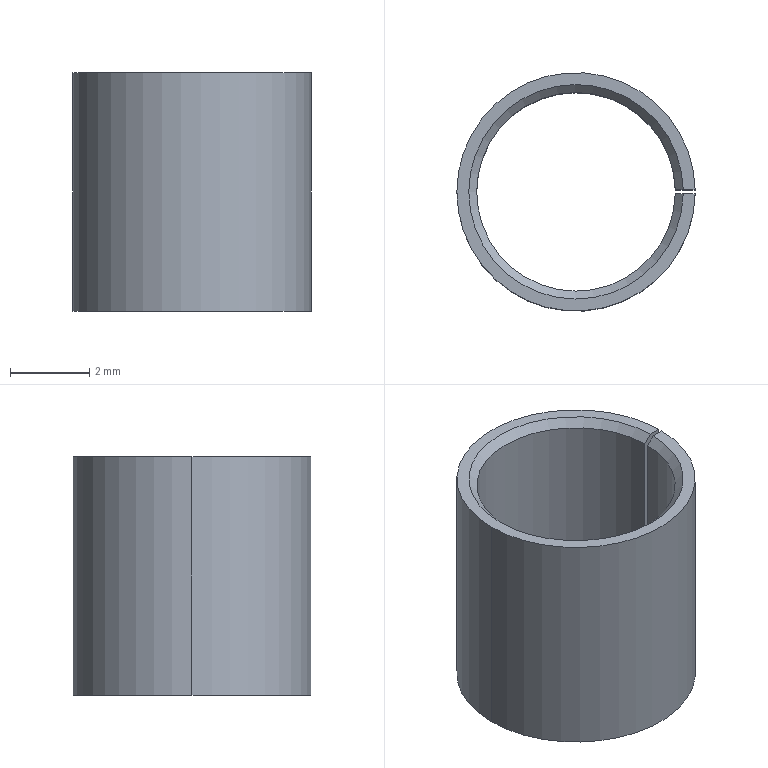Part | SolidWorks | features Chamfer 1, Extrusion 1, ICE 1 | 1 solid | 11 faces | box 6 x 6 x 6 mm | volume 50.895 mm3 | cylinder 4 | plane 4 | cone 3 | commonest cylinder face diameters 5 x2 6 x2
STEP:
#1=CARTESIAN_POINT('',(-2.5,0.,0.2));
#2=VERTEX_POINT('',#1);
#3=CARTESIAN_POINT('',(2.499,0.05,0.2));
#4=VERTEX_POINT('',#3);
#5=CARTESIAN_POINT('',(0.,0.,0.2));
#6=DIRECTION('',(0.,0.,-1.));
#7=DIRECTION('',(1.,0.,0.));
#8=AXIS2_PLACEMENT_3D('',#5,#6,#7);
#9=CIRCLE('',#8,2.5);
#10=EDGE_CURVE('',#2,#4,#9,.T.);
#11=ORIENTED_EDGE('',*,*,#10,.F.);
#12=CARTESIAN_POINT('',(-2.7,0.,0.));
#13=VERTEX_POINT('',#12);
#14=CARTESIAN_POINT('',(-2.7,0.,0.));
#15=DIRECTION('',(-0.7071,0.,-0.7071));
#16=VECTOR('',#15,1000.);
#17=LINE('',#14,#16);
#18=EDGE_CURVE('',#2,#13,#17,.T.);
#19=ORIENTED_EDGE('',*,*,#18,.T.);
#20=CARTESIAN_POINT('',(2.7,0.05,0.));
#21=VERTEX_POINT('',#20);
#22=CARTESIAN_POINT('',(0.,0.,0.));
#23=DIRECTION('',(0.,0.,1.));
#24=DIRECTION('',(1.,0.,0.));
#25=AXIS2_PLACEMENT_3D('',#22,#23,#24);
#26=CIRCLE('',#25,2.7);
#27=EDGE_CURVE('',#21,#13,#26,.T.);
#28=ORIENTED_EDGE('',*,*,#27,.F.);
#29=CARTESIAN_POINT('',(2.499,0.05,0.2));
#30=CARTESIAN_POINT('',(2.566,0.05,0.1333));
#31=CARTESIAN_POINT('',(2.633,0.05,0.06667));
#32=CARTESIAN_POINT('',(2.7,0.05,0.));
#33=B_SPLINE_CURVE_WITH_KNOTS('',3,(#29,#30,#31,#32),.UNSPECIFIED.,.F.,.F.,(4,4),(0.002926,0.003209),.UNSPECIFIED.);
#34=EDGE_CURVE('',#4,#21,#33,.T.);
#35=ORIENTED_EDGE('',*,*,#34,.F.);
#36=EDGE_LOOP('',(#11,#19,#28,#35));
#37=FACE_OUTER_BOUND('',#36,.T.);
#38=CARTESIAN_POINT('',(0.,0.,0.));
#39=DIRECTION('',(0.,0.,-1.));
#40=DIRECTION('',(-1.,0.,0.));
#41=AXIS2_PLACEMENT_3D('',#38,#39,#40);
#42=CONICAL_SURFACE('',#41,2.7,0.7854);
#43=ADVANCED_FACE('',(#37),#42,.F.);
#44=CARTESIAN_POINT('',(2.499,0.05,5.8));
#45=VERTEX_POINT('',#44);
#46=CARTESIAN_POINT('',(-2.5,0.,5.8));
#47=VERTEX_POINT('',#46);
#48=CARTESIAN_POINT('',(0.,0.,5.8));
#49=DIRECTION('',(0.,0.,1.));
#50=DIRECTION('',(1.,0.,0.));
#51=AXIS2_PLACEMENT_3D('',#48,#49,#50);
#52=CIRCLE('',#51,2.5);
#53=EDGE_CURVE('',#45,#47,#52,.T.);
#54=ORIENTED_EDGE('',*,*,#53,.T.);
#55=CARTESIAN_POINT('',(-2.5,0.,6.));
#56=DIRECTION('',(0.,0.,-1.));
#57=VECTOR('',#56,1000.);
#58=LINE('',#55,#57);
#59=EDGE_CURVE('',#47,#2,#58,.T.);
#60=ORIENTED_EDGE('',*,*,#59,.T.);
#61=ORIENTED_EDGE('',*,*,#10,.T.);
#62=CARTESIAN_POINT('',(2.499,0.05,6.));
#63=DIRECTION('',(0.,0.,-1.));
#64=VECTOR('',#63,1000.);
#65=LINE('',#62,#64);
#66=EDGE_CURVE('',#45,#4,#65,.T.);
#67=ORIENTED_EDGE('',*,*,#66,.F.);
#68=EDGE_LOOP('',(#54,#60,#61,#67));
#69=FACE_OUTER_BOUND('',#68,.T.);
#70=CARTESIAN_POINT('',(0.,0.,6.));
#71=DIRECTION('',(0.,0.,-1.));
#72=DIRECTION('',(-1.,0.,0.));
#73=AXIS2_PLACEMENT_3D('',#70,#71,#72);
#74=CYLINDRICAL_SURFACE('',#73,2.5);
#75=ADVANCED_FACE('',(#69),#74,.F.);
#76=CARTESIAN_POINT('',(-3.,0.,6.));
#77=VERTEX_POINT('',#76);
#78=CARTESIAN_POINT('',(3.,-0.05,6.));
#79=VERTEX_POINT('',#78);
#80=CARTESIAN_POINT('',(0.,0.,6.));
#81=DIRECTION('',(0.,0.,1.));
#82=DIRECTION('',(1.,0.,0.));
#83=AXIS2_PLACEMENT_3D('',#80,#81,#82);
#84=CIRCLE('',#83,3.);
#85=EDGE_CURVE('',#77,#79,#84,.T.);
#86=ORIENTED_EDGE('',*,*,#85,.F.);
#87=CARTESIAN_POINT('',(-3.,0.,0.));
#88=VERTEX_POINT('',#87);
#89=CARTESIAN_POINT('',(-3.,0.,6.));
#90=DIRECTION('',(0.,0.,-1.));
#91=VECTOR('',#90,1000.);
#92=LINE('',#89,#91);
#93=EDGE_CURVE('',#77,#88,#92,.T.);
#94=ORIENTED_EDGE('',*,*,#93,.T.);
#95=CARTESIAN_POINT('',(3.,-0.05,0.));
#96=VERTEX_POINT('',#95);
#97=CARTESIAN_POINT('',(0.,0.,0.));
#98=DIRECTION('',(0.,0.,1.));
#99=DIRECTION('',(1.,0.,0.));
#100=AXIS2_PLACEMENT_3D('',#97,#98,#99);
#101=CIRCLE('',#100,3.);
#102=EDGE_CURVE('',#88,#96,#101,.T.);
#103=ORIENTED_EDGE('',*,*,#102,.T.);
#104=CARTESIAN_POINT('',(3.,-0.05,6.));
#105=DIRECTION('',(0.,0.,1.));
#106=VECTOR('',#105,1000.);
#107=LINE('',#104,#106);
#108=EDGE_CURVE('',#96,#79,#107,.T.);
#109=ORIENTED_EDGE('',*,*,#108,.T.);
#110=EDGE_LOOP('',(#86,#94,#103,#109));
#111=FACE_OUTER_BOUND('',#110,.T.);
#112=CARTESIAN_POINT('',(0.,0.,6.));
#113=DIRECTION('',(0.,0.,-1.));
#114=DIRECTION('',(-1.,0.,0.));
#115=AXIS2_PLACEMENT_3D('',#112,#113,#114);
#116=CYLINDRICAL_SURFACE('',#115,3.);
#117=ADVANCED_FACE('',(#111),#116,.T.);
#118=CARTESIAN_POINT('',(2.7,-0.05,6.));
#119=VERTEX_POINT('',#118);
#120=CARTESIAN_POINT('',(0.6418,-0.05,6.));
#121=DIRECTION('',(1.,0.,0.));
#122=VECTOR('',#121,1000.);
#123=LINE('',#120,#122);
#124=EDGE_CURVE('',#119,#79,#123,.T.);
#125=ORIENTED_EDGE('',*,*,#124,.F.);
#126=CARTESIAN_POINT('',(2.7,0.05,6.));
#127=VERTEX_POINT('',#126);
#128=CARTESIAN_POINT('',(0.,0.,6.));
#129=DIRECTION('',(0.,0.,-1.));
#130=DIRECTION('',(1.,0.,0.));
#131=AXIS2_PLACEMENT_3D('',#128,#129,#130);
#132=CIRCLE('',#131,2.7);
#133=EDGE_CURVE('',#119,#127,#132,.T.);
#134=ORIENTED_EDGE('',*,*,#133,.T.);
#135=CARTESIAN_POINT('',(3.,0.05,6.));
#136=VERTEX_POINT('',#135);
#137=CARTESIAN_POINT('',(0.6418,0.05,6.));
#138=DIRECTION('',(-1.,0.,0.));
#139=VECTOR('',#138,1000.);
#140=LINE('',#137,#139);
#141=EDGE_CURVE('',#136,#127,#140,.T.);
#142=ORIENTED_EDGE('',*,*,#141,.F.);
#143=CARTESIAN_POINT('',(0.,0.,6.));
#144=DIRECTION('',(0.,0.,1.));
#145=DIRECTION('',(1.,0.,0.));
#146=AXIS2_PLACEMENT_3D('',#143,#144,#145);
#147=CIRCLE('',#146,3.);
#148=EDGE_CURVE('',#136,#77,#147,.T.);
#149=ORIENTED_EDGE('',*,*,#148,.T.);
#150=ORIENTED_EDGE('',*,*,#85,.T.);
#151=EDGE_LOOP('',(#125,#134,#142,#149,#150));
#152=FACE_OUTER_BOUND('',#151,.T.);
#153=CARTESIAN_POINT('',(0.,0.,6.));
#154=DIRECTION('',(0.,0.,1.));
#155=DIRECTION('',(1.,0.,0.));
#156=AXIS2_PLACEMENT_3D('',#153,#154,#155);
#157=PLANE('',#156);
#158=ADVANCED_FACE('',(#152),#157,.T.);
#159=ORIENTED_EDGE('',*,*,#27,.T.);
#160=CARTESIAN_POINT('',(2.7,-0.05,0.));
#161=VERTEX_POINT('',#160);
#162=CARTESIAN_POINT('',(0.,0.,0.));
#163=DIRECTION('',(0.,0.,1.));
#164=DIRECTION('',(1.,0.,0.));
#165=AXIS2_PLACEMENT_3D('',#162,#163,#164);
#166=CIRCLE('',#165,2.7);
#167=EDGE_CURVE('',#13,#161,#166,.T.);
#168=ORIENTED_EDGE('',*,*,#167,.T.);
#169=CARTESIAN_POINT('',(0.6418,-0.05,0.));
#170=DIRECTION('',(1.,0.,0.));
#171=VECTOR('',#170,1000.);
#172=LINE('',#169,#171);
#173=EDGE_CURVE('',#161,#96,#172,.T.);
#174=ORIENTED_EDGE('',*,*,#173,.T.);
#175=ORIENTED_EDGE('',*,*,#102,.F.);
#176=CARTESIAN_POINT('',(3.,0.05,0.));
#177=VERTEX_POINT('',#176);
#178=CARTESIAN_POINT('',(0.,0.,0.));
#179=DIRECTION('',(0.,0.,1.));
#180=DIRECTION('',(1.,0.,0.));
#181=AXIS2_PLACEMENT_3D('',#178,#179,#180);
#182=CIRCLE('',#181,3.);
#183=EDGE_CURVE('',#177,#88,#182,.T.);
#184=ORIENTED_EDGE('',*,*,#183,.F.);
#185=CARTESIAN_POINT('',(0.6418,0.05,0.));
#186=DIRECTION('',(-1.,0.,0.));
#187=VECTOR('',#186,1000.);
#188=LINE('',#185,#187);
#189=EDGE_CURVE('',#177,#21,#188,.T.);
#190=ORIENTED_EDGE('',*,*,#189,.T.);
#191=EDGE_LOOP('',(#159,#168,#174,#175,#184,#190));
#192=FACE_OUTER_BOUND('',#191,.T.);
#193=CARTESIAN_POINT('',(0.,0.,0.));
#194=DIRECTION('',(0.,0.,1.));
#195=DIRECTION('',(1.,0.,0.));
#196=AXIS2_PLACEMENT_3D('',#193,#194,#195);
#197=PLANE('',#196);
#198=ADVANCED_FACE('',(#192),#197,.F.);
#199=ORIENTED_EDGE('',*,*,#93,.F.);
#200=ORIENTED_EDGE('',*,*,#148,.F.);
#201=CARTESIAN_POINT('',(3.,0.05,6.));
#202=DIRECTION('',(0.,0.,-1.));
#203=VECTOR('',#202,1000.);
#204=LINE('',#201,#203);
#205=EDGE_CURVE('',#136,#177,#204,.T.);
#206=ORIENTED_EDGE('',*,*,#205,.T.);
#207=ORIENTED_EDGE('',*,*,#183,.T.);
#208=EDGE_LOOP('',(#199,#200,#206,#207));
#209=FACE_OUTER_BOUND('',#208,.T.);
#210=CARTESIAN_POINT('',(0.,0.,6.));
#211=DIRECTION('',(0.,0.,-1.));
#212=DIRECTION('',(-1.,0.,0.));
#213=AXIS2_PLACEMENT_3D('',#210,#211,#212);
#214=CYLINDRICAL_SURFACE('',#213,3.);
#215=ADVANCED_FACE('',(#209),#214,.T.);
#216=ORIENTED_EDGE('',*,*,#59,.F.);
#217=CARTESIAN_POINT('',(2.499,-0.05,5.8));
#218=VERTEX_POINT('',#217);
#219=CARTESIAN_POINT('',(0.,0.,5.8));
#220=DIRECTION('',(0.,0.,1.));
#221=DIRECTION('',(1.,0.,0.));
#222=AXIS2_PLACEMENT_3D('',#219,#220,#221);
#223=CIRCLE('',#222,2.5);
#224=EDGE_CURVE('',#47,#218,#223,.T.);
#225=ORIENTED_EDGE('',*,*,#224,.T.);
#226=CARTESIAN_POINT('',(2.499,-0.05,0.2));
#227=VERTEX_POINT('',#226);
#228=CARTESIAN_POINT('',(2.499,-0.05,6.));
#229=DIRECTION('',(0.,0.,1.));
#230=VECTOR('',#229,1000.);
#231=LINE('',#228,#230);
#232=EDGE_CURVE('',#227,#218,#231,.T.);
#233=ORIENTED_EDGE('',*,*,#232,.F.);
#234=CARTESIAN_POINT('',(0.,0.,0.2));
#235=DIRECTION('',(0.,0.,-1.));
#236=DIRECTION('',(1.,0.,0.));
#237=AXIS2_PLACEMENT_3D('',#234,#235,#236);
#238=CIRCLE('',#237,2.5);
#239=EDGE_CURVE('',#227,#2,#238,.T.);
#240=ORIENTED_EDGE('',*,*,#239,.T.);
#241=EDGE_LOOP('',(#216,#225,#233,#240));
#242=FACE_OUTER_BOUND('',#241,.T.);
#243=CARTESIAN_POINT('',(0.,0.,6.));
#244=DIRECTION('',(0.,0.,-1.));
#245=DIRECTION('',(-1.,0.,0.));
#246=AXIS2_PLACEMENT_3D('',#243,#244,#245);
#247=CYLINDRICAL_SURFACE('',#246,2.5);
#248=ADVANCED_FACE('',(#242),#247,.F.);
#249=ORIENTED_EDGE('',*,*,#18,.F.);
#250=ORIENTED_EDGE('',*,*,#239,.F.);
#251=CARTESIAN_POINT('',(2.7,-0.05,0.));
#252=CARTESIAN_POINT('',(2.633,-0.05,0.06667));
#253=CARTESIAN_POINT('',(2.566,-0.05,0.1333));
#254=CARTESIAN_POINT('',(2.499,-0.05,0.2));
#255=B_SPLINE_CURVE_WITH_KNOTS('',3,(#251,#252,#253,#254),.UNSPECIFIED.,.F.,.F.,(4,4),(0.002925,0.003208),.UNSPECIFIED.);
#256=EDGE_CURVE('',#161,#227,#255,.T.);
#257=ORIENTED_EDGE('',*,*,#256,.F.);
#258=ORIENTED_EDGE('',*,*,#167,.F.);
#259=EDGE_LOOP('',(#249,#250,#257,#258));
#260=FACE_OUTER_BOUND('',#259,.T.);
#261=CARTESIAN_POINT('',(0.,0.,0.));
#262=DIRECTION('',(0.,0.,-1.));
#263=DIRECTION('',(-1.,0.,0.));
#264=AXIS2_PLACEMENT_3D('',#261,#262,#263);
#265=CONICAL_SURFACE('',#264,2.7,0.7854);
#266=ADVANCED_FACE('',(#260),#265,.F.);
#267=CARTESIAN_POINT('',(2.499,-0.05,5.8));
#268=CARTESIAN_POINT('',(2.566,-0.05,5.867));
#269=CARTESIAN_POINT('',(2.633,-0.05,5.933));
#270=CARTESIAN_POINT('',(2.7,-0.05,6.));
#271=B_SPLINE_CURVE_WITH_KNOTS('',3,(#267,#268,#269,#270),.UNSPECIFIED.,.F.,.F.,(4,4),(0.002926,0.003209),.UNSPECIFIED.);
#272=EDGE_CURVE('',#218,#119,#271,.T.);
#273=ORIENTED_EDGE('',*,*,#272,.F.);
#274=ORIENTED_EDGE('',*,*,#224,.F.);
#275=ORIENTED_EDGE('',*,*,#53,.F.);
#276=CARTESIAN_POINT('',(2.7,0.05,6.));
#277=CARTESIAN_POINT('',(2.633,0.05,5.933));
#278=CARTESIAN_POINT('',(2.566,0.05,5.867));
#279=CARTESIAN_POINT('',(2.499,0.05,5.8));
#280=B_SPLINE_CURVE_WITH_KNOTS('',3,(#276,#277,#278,#279),.UNSPECIFIED.,.F.,.F.,(4,4),(0.002925,0.003208),.UNSPECIFIED.);
#281=EDGE_CURVE('',#127,#45,#280,.T.);
#282=ORIENTED_EDGE('',*,*,#281,.F.);
#283=ORIENTED_EDGE('',*,*,#133,.F.);
#284=EDGE_LOOP('',(#273,#274,#275,#282,#283));
#285=FACE_OUTER_BOUND('',#284,.T.);
#286=CARTESIAN_POINT('',(0.,0.,5.8));
#287=DIRECTION('',(0.,0.,1.));
#288=DIRECTION('',(1.,0.,0.));
#289=AXIS2_PLACEMENT_3D('',#286,#287,#288);
#290=CONICAL_SURFACE('',#289,2.5,0.7854);
#291=ADVANCED_FACE('',(#285),#290,.F.);
#292=ORIENTED_EDGE('',*,*,#141,.T.);
#293=ORIENTED_EDGE('',*,*,#281,.T.);
#294=ORIENTED_EDGE('',*,*,#66,.T.);
#295=ORIENTED_EDGE('',*,*,#34,.T.);
#296=ORIENTED_EDGE('',*,*,#189,.F.);
#297=ORIENTED_EDGE('',*,*,#205,.F.);
#298=EDGE_LOOP('',(#292,#293,#294,#295,#296,#297));
#299=FACE_OUTER_BOUND('',#298,.T.);
#300=CARTESIAN_POINT('',(0.6418,0.05,0.));
#301=DIRECTION('',(0.,1.,0.));
#302=DIRECTION('',(0.,0.,1.));
#303=AXIS2_PLACEMENT_3D('',#300,#301,#302);
#304=PLANE('',#303);
#305=ADVANCED_FACE('',(#299),#304,.F.);
#306=ORIENTED_EDGE('',*,*,#173,.F.);
#307=ORIENTED_EDGE('',*,*,#256,.T.);
#308=ORIENTED_EDGE('',*,*,#232,.T.);
#309=ORIENTED_EDGE('',*,*,#272,.T.);
#310=ORIENTED_EDGE('',*,*,#124,.T.);
#311=ORIENTED_EDGE('',*,*,#108,.F.);
#312=EDGE_LOOP('',(#306,#307,#308,#309,#310,#311));
#313=FACE_OUTER_BOUND('',#312,.T.);
#314=CARTESIAN_POINT('',(0.6418,-0.05,0.));
#315=DIRECTION('',(0.,-1.,0.));
#316=DIRECTION('',(0.,0.,-1.));
#317=AXIS2_PLACEMENT_3D('',#314,#315,#316);
#318=PLANE('',#317);
#319=ADVANCED_FACE('',(#313),#318,.F.);
#320=CLOSED_SHELL('',(#43,#75,#117,#158,#198,#215,#248,#266,#291,#305,#319));
#321=MANIFOLD_SOLID_BREP('',#320);
#322=CARTESIAN_POINT('',(0.,0.,0.));
#323=DIRECTION('',(0.,0.,1.));
#324=DIRECTION('',(1.,0.,0.));
#325=AXIS2_PLACEMENT_3D('',#322,#323,#324);
#326=(LENGTH_UNIT()NAMED_UNIT(*)SI_UNIT(.MILLI.,.METRE.));
#327=UNCERTAINTY_MEASURE_WITH_UNIT(LENGTH_MEASURE(0.00001),#326,'','');
#328=(NAMED_UNIT(*)PLANE_ANGLE_UNIT()SI_UNIT($,.RADIAN.));
#329=(NAMED_UNIT(*)SI_UNIT($,.STERADIAN.)SOLID_ANGLE_UNIT());
#330=(GEOMETRIC_REPRESENTATION_CONTEXT(3)GLOBAL_UNCERTAINTY_ASSIGNED_CONTEXT((#327))GLOBAL_UNIT_ASSIGNED_CONTEXT((#326,#328,#329))REPRESENTATION_CONTEXT('',''));
#331=ADVANCED_BREP_SHAPE_REPRESENTATION('',(#321,#325),#330);